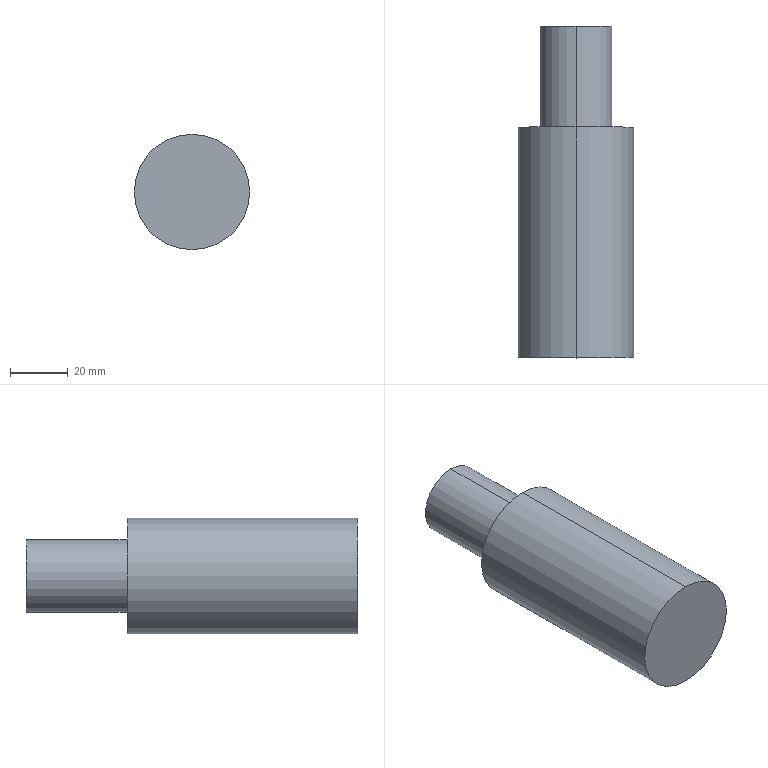Part | SolidWorks | features Revolution 1 | 1 solid | 13 faces | box 40 x 115 x 40 mm | volume 61163 mm3 | cylinder 8 | plane 5 | commonest cylinder face diameters 15 x2 25 x2 30 x2 40 x2
STEP:
#1=CARTESIAN_POINT('',(-73.129,-137.973,-15.));
#2=VERTEX_POINT('',#1);
#3=CARTESIAN_POINT('',(-73.129,-137.973,15.));
#4=VERTEX_POINT('',#3);
#5=CARTESIAN_POINT('',(-73.129,-137.973,0.));
#6=DIRECTION('',(0.,1.,0.));
#7=DIRECTION('',(0.,0.,1.));
#8=AXIS2_PLACEMENT_3D('',#5,#6,#7);
#9=CIRCLE('',#8,15.);
#10=EDGE_CURVE('',#2,#4,#9,.T.);
#11=ORIENTED_EDGE('',*,*,#10,.F.);
#12=CARTESIAN_POINT('',(-73.129,-67.973,-15.));
#13=VERTEX_POINT('',#12);
#14=CARTESIAN_POINT('',(-73.129,-60.,-15.));
#15=DIRECTION('',(0.,1.,0.));
#16=VECTOR('',#15,1000.);
#17=LINE('',#14,#16);
#18=EDGE_CURVE('',#2,#13,#17,.T.);
#19=ORIENTED_EDGE('',*,*,#18,.T.);
#20=CARTESIAN_POINT('',(-73.129,-67.973,15.));
#21=VERTEX_POINT('',#20);
#22=CARTESIAN_POINT('',(-73.129,-67.973,0.));
#23=DIRECTION('',(0.,1.,0.));
#24=DIRECTION('',(0.,0.,1.));
#25=AXIS2_PLACEMENT_3D('',#22,#23,#24);
#26=CIRCLE('',#25,15.);
#27=EDGE_CURVE('',#13,#21,#26,.T.);
#28=ORIENTED_EDGE('',*,*,#27,.T.);
#29=CARTESIAN_POINT('',(-73.129,-60.,15.));
#30=DIRECTION('',(0.,1.,0.));
#31=VECTOR('',#30,1000.);
#32=LINE('',#29,#31);
#33=EDGE_CURVE('',#4,#21,#32,.T.);
#34=ORIENTED_EDGE('',*,*,#33,.F.);
#35=EDGE_LOOP('',(#11,#19,#28,#34));
#36=FACE_OUTER_BOUND('',#35,.T.);
#37=CARTESIAN_POINT('',(-73.129,-60.,0.));
#38=DIRECTION('',(0.,1.,0.));
#39=DIRECTION('',(0.,0.,1.));
#40=AXIS2_PLACEMENT_3D('',#37,#38,#39);
#41=CYLINDRICAL_SURFACE('',#40,15.);
#42=ADVANCED_FACE('',(#36),#41,.F.);
#43=CARTESIAN_POINT('',(-73.129,-142.973,20.));
#44=VERTEX_POINT('',#43);
#45=CARTESIAN_POINT('',(-73.129,-142.973,-20.));
#46=VERTEX_POINT('',#45);
#47=CARTESIAN_POINT('',(-73.129,-142.973,0.));
#48=DIRECTION('',(0.,1.,0.));
#49=DIRECTION('',(0.,0.,1.));
#50=AXIS2_PLACEMENT_3D('',#47,#48,#49);
#51=CIRCLE('',#50,20.);
#52=EDGE_CURVE('',#44,#46,#51,.T.);
#53=ORIENTED_EDGE('',*,*,#52,.T.);
#54=CARTESIAN_POINT('',(-73.129,-62.973,-20.));
#55=VERTEX_POINT('',#54);
#56=CARTESIAN_POINT('',(-73.129,-60.,-20.));
#57=DIRECTION('',(0.,1.,0.));
#58=VECTOR('',#57,1000.);
#59=LINE('',#56,#58);
#60=EDGE_CURVE('',#46,#55,#59,.T.);
#61=ORIENTED_EDGE('',*,*,#60,.T.);
#62=CARTESIAN_POINT('',(-73.129,-62.973,20.));
#63=VERTEX_POINT('',#62);
#64=CARTESIAN_POINT('',(-73.129,-62.973,0.));
#65=DIRECTION('',(0.,1.,0.));
#66=DIRECTION('',(0.,0.,1.));
#67=AXIS2_PLACEMENT_3D('',#64,#65,#66);
#68=CIRCLE('',#67,20.);
#69=EDGE_CURVE('',#63,#55,#68,.T.);
#70=ORIENTED_EDGE('',*,*,#69,.F.);
#71=CARTESIAN_POINT('',(-73.129,-60.,20.));
#72=DIRECTION('',(0.,1.,0.));
#73=VECTOR('',#72,1000.);
#74=LINE('',#71,#73);
#75=EDGE_CURVE('',#44,#63,#74,.T.);
#76=ORIENTED_EDGE('',*,*,#75,.F.);
#77=EDGE_LOOP('',(#53,#61,#70,#76));
#78=FACE_OUTER_BOUND('',#77,.T.);
#79=CARTESIAN_POINT('',(-73.129,-60.,0.));
#80=DIRECTION('',(0.,1.,0.));
#81=DIRECTION('',(0.,0.,1.));
#82=AXIS2_PLACEMENT_3D('',#79,#80,#81);
#83=CYLINDRICAL_SURFACE('',#82,20.);
#84=ADVANCED_FACE('',(#78),#83,.T.);
#85=CARTESIAN_POINT('',(-73.129,-62.973,12.5));
#86=VERTEX_POINT('',#85);
#87=CARTESIAN_POINT('',(-73.129,-62.973,-12.5));
#88=VERTEX_POINT('',#87);
#89=CARTESIAN_POINT('',(-73.129,-62.973,0.));
#90=DIRECTION('',(0.,1.,0.));
#91=DIRECTION('',(0.,0.,1.));
#92=AXIS2_PLACEMENT_3D('',#89,#90,#91);
#93=CIRCLE('',#92,12.5);
#94=EDGE_CURVE('',#86,#88,#93,.T.);
#95=ORIENTED_EDGE('',*,*,#94,.T.);
#96=CARTESIAN_POINT('',(-73.129,-27.973,-12.5));
#97=VERTEX_POINT('',#96);
#98=CARTESIAN_POINT('',(-73.129,-60.,-12.5));
#99=DIRECTION('',(0.,1.,0.));
#100=VECTOR('',#99,1000.);
#101=LINE('',#98,#100);
#102=EDGE_CURVE('',#88,#97,#101,.T.);
#103=ORIENTED_EDGE('',*,*,#102,.T.);
#104=CARTESIAN_POINT('',(-73.129,-27.973,12.5));
#105=VERTEX_POINT('',#104);
#106=CARTESIAN_POINT('',(-73.129,-27.973,0.));
#107=DIRECTION('',(0.,1.,0.));
#108=DIRECTION('',(0.,0.,1.));
#109=AXIS2_PLACEMENT_3D('',#106,#107,#108);
#110=CIRCLE('',#109,12.5);
#111=EDGE_CURVE('',#105,#97,#110,.T.);
#112=ORIENTED_EDGE('',*,*,#111,.F.);
#113=CARTESIAN_POINT('',(-73.129,-60.,12.5));
#114=DIRECTION('',(0.,1.,0.));
#115=VECTOR('',#114,1000.);
#116=LINE('',#113,#115);
#117=EDGE_CURVE('',#86,#105,#116,.T.);
#118=ORIENTED_EDGE('',*,*,#117,.F.);
#119=EDGE_LOOP('',(#95,#103,#112,#118));
#120=FACE_OUTER_BOUND('',#119,.T.);
#121=CARTESIAN_POINT('',(-73.129,-60.,0.));
#122=DIRECTION('',(0.,1.,0.));
#123=DIRECTION('',(0.,0.,1.));
#124=AXIS2_PLACEMENT_3D('',#121,#122,#123);
#125=CYLINDRICAL_SURFACE('',#124,12.5);
#126=ADVANCED_FACE('',(#120),#125,.T.);
#127=CARTESIAN_POINT('',(-73.129,-67.973,-7.5));
#128=VERTEX_POINT('',#127);
#129=CARTESIAN_POINT('',(-73.129,-67.973,7.5));
#130=VERTEX_POINT('',#129);
#131=CARTESIAN_POINT('',(-73.129,-67.973,0.));
#132=DIRECTION('',(0.,1.,0.));
#133=DIRECTION('',(0.,0.,1.));
#134=AXIS2_PLACEMENT_3D('',#131,#132,#133);
#135=CIRCLE('',#134,7.5);
#136=EDGE_CURVE('',#128,#130,#135,.T.);
#137=ORIENTED_EDGE('',*,*,#136,.F.);
#138=CARTESIAN_POINT('',(-73.129,-27.973,-7.5));
#139=VERTEX_POINT('',#138);
#140=CARTESIAN_POINT('',(-73.129,-60.,-7.5));
#141=DIRECTION('',(0.,1.,0.));
#142=VECTOR('',#141,1000.);
#143=LINE('',#140,#142);
#144=EDGE_CURVE('',#128,#139,#143,.T.);
#145=ORIENTED_EDGE('',*,*,#144,.T.);
#146=CARTESIAN_POINT('',(-73.129,-27.973,7.5));
#147=VERTEX_POINT('',#146);
#148=CARTESIAN_POINT('',(-73.129,-27.973,0.));
#149=DIRECTION('',(0.,1.,0.));
#150=DIRECTION('',(0.,0.,1.));
#151=AXIS2_PLACEMENT_3D('',#148,#149,#150);
#152=CIRCLE('',#151,7.5);
#153=EDGE_CURVE('',#139,#147,#152,.T.);
#154=ORIENTED_EDGE('',*,*,#153,.T.);
#155=CARTESIAN_POINT('',(-73.129,-60.,7.5));
#156=DIRECTION('',(0.,1.,0.));
#157=VECTOR('',#156,1000.);
#158=LINE('',#155,#157);
#159=EDGE_CURVE('',#130,#147,#158,.T.);
#160=ORIENTED_EDGE('',*,*,#159,.F.);
#161=EDGE_LOOP('',(#137,#145,#154,#160));
#162=FACE_OUTER_BOUND('',#161,.T.);
#163=CARTESIAN_POINT('',(-73.129,-60.,0.));
#164=DIRECTION('',(0.,1.,0.));
#165=DIRECTION('',(0.,0.,1.));
#166=AXIS2_PLACEMENT_3D('',#163,#164,#165);
#167=CYLINDRICAL_SURFACE('',#166,7.5);
#168=ADVANCED_FACE('',(#162),#167,.F.);
#169=ORIENTED_EDGE('',*,*,#144,.F.);
#170=CARTESIAN_POINT('',(-73.129,-67.973,0.));
#171=DIRECTION('',(0.,1.,0.));
#172=DIRECTION('',(0.,0.,1.));
#173=AXIS2_PLACEMENT_3D('',#170,#171,#172);
#174=CIRCLE('',#173,7.5);
#175=EDGE_CURVE('',#130,#128,#174,.T.);
#176=ORIENTED_EDGE('',*,*,#175,.F.);
#177=ORIENTED_EDGE('',*,*,#159,.T.);
#178=CARTESIAN_POINT('',(-73.129,-27.973,0.));
#179=DIRECTION('',(0.,1.,0.));
#180=DIRECTION('',(0.,0.,1.));
#181=AXIS2_PLACEMENT_3D('',#178,#179,#180);
#182=CIRCLE('',#181,7.5);
#183=EDGE_CURVE('',#147,#139,#182,.T.);
#184=ORIENTED_EDGE('',*,*,#183,.T.);
#185=EDGE_LOOP('',(#169,#176,#177,#184));
#186=FACE_OUTER_BOUND('',#185,.T.);
#187=CARTESIAN_POINT('',(-73.129,-60.,0.));
#188=DIRECTION('',(0.,1.,0.));
#189=DIRECTION('',(0.,0.,1.));
#190=AXIS2_PLACEMENT_3D('',#187,#188,#189);
#191=CYLINDRICAL_SURFACE('',#190,7.5);
#192=ADVANCED_FACE('',(#186),#191,.F.);
#193=ORIENTED_EDGE('',*,*,#183,.F.);
#194=ORIENTED_EDGE('',*,*,#153,.F.);
#195=EDGE_LOOP('',(#193,#194));
#196=FACE_BOUND('',#195,.T.);
#197=ORIENTED_EDGE('',*,*,#111,.T.);
#198=CARTESIAN_POINT('',(-73.129,-27.973,0.));
#199=DIRECTION('',(0.,1.,0.));
#200=DIRECTION('',(0.,0.,1.));
#201=AXIS2_PLACEMENT_3D('',#198,#199,#200);
#202=CIRCLE('',#201,12.5);
#203=EDGE_CURVE('',#97,#105,#202,.T.);
#204=ORIENTED_EDGE('',*,*,#203,.T.);
#205=EDGE_LOOP('',(#197,#204));
#206=FACE_OUTER_BOUND('',#205,.T.);
#207=CARTESIAN_POINT('',(-65.629,-27.973,0.));
#208=DIRECTION('',(0.,-1.,0.));
#209=DIRECTION('',(0.,0.,-1.));
#210=AXIS2_PLACEMENT_3D('',#207,#208,#209);
#211=PLANE('',#210);
#212=ADVANCED_FACE('',(#196,#206),#211,.F.);
#213=ORIENTED_EDGE('',*,*,#102,.F.);
#214=CARTESIAN_POINT('',(-73.129,-62.973,0.));
#215=DIRECTION('',(0.,1.,0.));
#216=DIRECTION('',(0.,0.,1.));
#217=AXIS2_PLACEMENT_3D('',#214,#215,#216);
#218=CIRCLE('',#217,12.5);
#219=EDGE_CURVE('',#88,#86,#218,.T.);
#220=ORIENTED_EDGE('',*,*,#219,.T.);
#221=ORIENTED_EDGE('',*,*,#117,.T.);
#222=ORIENTED_EDGE('',*,*,#203,.F.);
#223=EDGE_LOOP('',(#213,#220,#221,#222));
#224=FACE_OUTER_BOUND('',#223,.T.);
#225=CARTESIAN_POINT('',(-73.129,-60.,0.));
#226=DIRECTION('',(0.,1.,0.));
#227=DIRECTION('',(0.,0.,1.));
#228=AXIS2_PLACEMENT_3D('',#225,#226,#227);
#229=CYLINDRICAL_SURFACE('',#228,12.5);
#230=ADVANCED_FACE('',(#224),#229,.T.);
#231=ORIENTED_EDGE('',*,*,#94,.F.);
#232=ORIENTED_EDGE('',*,*,#219,.F.);
#233=EDGE_LOOP('',(#231,#232));
#234=FACE_BOUND('',#233,.T.);
#235=ORIENTED_EDGE('',*,*,#69,.T.);
#236=CARTESIAN_POINT('',(-73.129,-62.973,0.));
#237=DIRECTION('',(0.,1.,0.));
#238=DIRECTION('',(0.,0.,1.));
#239=AXIS2_PLACEMENT_3D('',#236,#237,#238);
#240=CIRCLE('',#239,20.);
#241=EDGE_CURVE('',#55,#63,#240,.T.);
#242=ORIENTED_EDGE('',*,*,#241,.T.);
#243=EDGE_LOOP('',(#235,#242));
#244=FACE_OUTER_BOUND('',#243,.T.);
#245=CARTESIAN_POINT('',(-60.629,-62.973,0.));
#246=DIRECTION('',(0.,-1.,0.));
#247=DIRECTION('',(0.,0.,-1.));
#248=AXIS2_PLACEMENT_3D('',#245,#246,#247);
#249=PLANE('',#248);
#250=ADVANCED_FACE('',(#234,#244),#249,.F.);
#251=ORIENTED_EDGE('',*,*,#60,.F.);
#252=CARTESIAN_POINT('',(-73.129,-142.973,0.));
#253=DIRECTION('',(0.,1.,0.));
#254=DIRECTION('',(0.,0.,1.));
#255=AXIS2_PLACEMENT_3D('',#252,#253,#254);
#256=CIRCLE('',#255,20.);
#257=EDGE_CURVE('',#46,#44,#256,.T.);
#258=ORIENTED_EDGE('',*,*,#257,.T.);
#259=ORIENTED_EDGE('',*,*,#75,.T.);
#260=ORIENTED_EDGE('',*,*,#241,.F.);
#261=EDGE_LOOP('',(#251,#258,#259,#260));
#262=FACE_OUTER_BOUND('',#261,.T.);
#263=CARTESIAN_POINT('',(-73.129,-60.,0.));
#264=DIRECTION('',(0.,1.,0.));
#265=DIRECTION('',(0.,0.,1.));
#266=AXIS2_PLACEMENT_3D('',#263,#264,#265);
#267=CYLINDRICAL_SURFACE('',#266,20.);
#268=ADVANCED_FACE('',(#262),#267,.T.);
#269=ORIENTED_EDGE('',*,*,#52,.F.);
#270=ORIENTED_EDGE('',*,*,#257,.F.);
#271=EDGE_LOOP('',(#269,#270));
#272=FACE_OUTER_BOUND('',#271,.T.);
#273=CARTESIAN_POINT('',(-53.129,-142.973,0.));
#274=DIRECTION('',(0.,1.,0.));
#275=DIRECTION('',(0.,0.,1.));
#276=AXIS2_PLACEMENT_3D('',#273,#274,#275);
#277=PLANE('',#276);
#278=ADVANCED_FACE('',(#272),#277,.F.);
#279=CARTESIAN_POINT('',(-73.129,-137.973,0.));
#280=DIRECTION('',(0.,1.,0.));
#281=DIRECTION('',(0.,0.,1.));
#282=AXIS2_PLACEMENT_3D('',#279,#280,#281);
#283=CIRCLE('',#282,15.);
#284=EDGE_CURVE('',#4,#2,#283,.T.);
#285=ORIENTED_EDGE('',*,*,#284,.T.);
#286=ORIENTED_EDGE('',*,*,#10,.T.);
#287=EDGE_LOOP('',(#285,#286));
#288=FACE_OUTER_BOUND('',#287,.T.);
#289=CARTESIAN_POINT('',(-73.129,-137.973,0.));
#290=DIRECTION('',(0.,-1.,0.));
#291=DIRECTION('',(0.,0.,-1.));
#292=AXIS2_PLACEMENT_3D('',#289,#290,#291);
#293=PLANE('',#292);
#294=ADVANCED_FACE('',(#288),#293,.F.);
#295=ORIENTED_EDGE('',*,*,#18,.F.);
#296=ORIENTED_EDGE('',*,*,#284,.F.);
#297=ORIENTED_EDGE('',*,*,#33,.T.);
#298=CARTESIAN_POINT('',(-73.129,-67.973,0.));
#299=DIRECTION('',(0.,1.,0.));
#300=DIRECTION('',(0.,0.,1.));
#301=AXIS2_PLACEMENT_3D('',#298,#299,#300);
#302=CIRCLE('',#301,15.);
#303=EDGE_CURVE('',#21,#13,#302,.T.);
#304=ORIENTED_EDGE('',*,*,#303,.T.);
#305=EDGE_LOOP('',(#295,#296,#297,#304));
#306=FACE_OUTER_BOUND('',#305,.T.);
#307=CARTESIAN_POINT('',(-73.129,-60.,0.));
#308=DIRECTION('',(0.,1.,0.));
#309=DIRECTION('',(0.,0.,1.));
#310=AXIS2_PLACEMENT_3D('',#307,#308,#309);
#311=CYLINDRICAL_SURFACE('',#310,15.);
#312=ADVANCED_FACE('',(#306),#311,.F.);
#313=ORIENTED_EDGE('',*,*,#303,.F.);
#314=ORIENTED_EDGE('',*,*,#27,.F.);
#315=EDGE_LOOP('',(#313,#314));
#316=FACE_OUTER_BOUND('',#315,.T.);
#317=ORIENTED_EDGE('',*,*,#175,.T.);
#318=ORIENTED_EDGE('',*,*,#136,.T.);
#319=EDGE_LOOP('',(#317,#318));
#320=FACE_BOUND('',#319,.T.);
#321=CARTESIAN_POINT('',(-58.129,-67.973,0.));
#322=DIRECTION('',(0.,1.,0.));
#323=DIRECTION('',(0.,0.,1.));
#324=AXIS2_PLACEMENT_3D('',#321,#322,#323);
#325=PLANE('',#324);
#326=ADVANCED_FACE('',(#316,#320),#325,.F.);
#327=CLOSED_SHELL('',(#42,#84,#126,#168,#192,#212,#230,#250,#268,#278,#294,#312,#326));
#328=MANIFOLD_SOLID_BREP('',#327);
#329=CARTESIAN_POINT('',(0.,0.,0.));
#330=DIRECTION('',(0.,0.,1.));
#331=DIRECTION('',(1.,0.,0.));
#332=AXIS2_PLACEMENT_3D('',#329,#330,#331);
#333=(LENGTH_UNIT()NAMED_UNIT(*)SI_UNIT(.MILLI.,.METRE.));
#334=UNCERTAINTY_MEASURE_WITH_UNIT(LENGTH_MEASURE(0.00001),#333,'','');
#335=(NAMED_UNIT(*)PLANE_ANGLE_UNIT()SI_UNIT($,.RADIAN.));
#336=(NAMED_UNIT(*)SI_UNIT($,.STERADIAN.)SOLID_ANGLE_UNIT());
#337=(GEOMETRIC_REPRESENTATION_CONTEXT(3)GLOBAL_UNCERTAINTY_ASSIGNED_CONTEXT((#334))GLOBAL_UNIT_ASSIGNED_CONTEXT((#333,#335,#336))REPRESENTATION_CONTEXT('',''));
#338=ADVANCED_BREP_SHAPE_REPRESENTATION('',(#328,#332),#337);